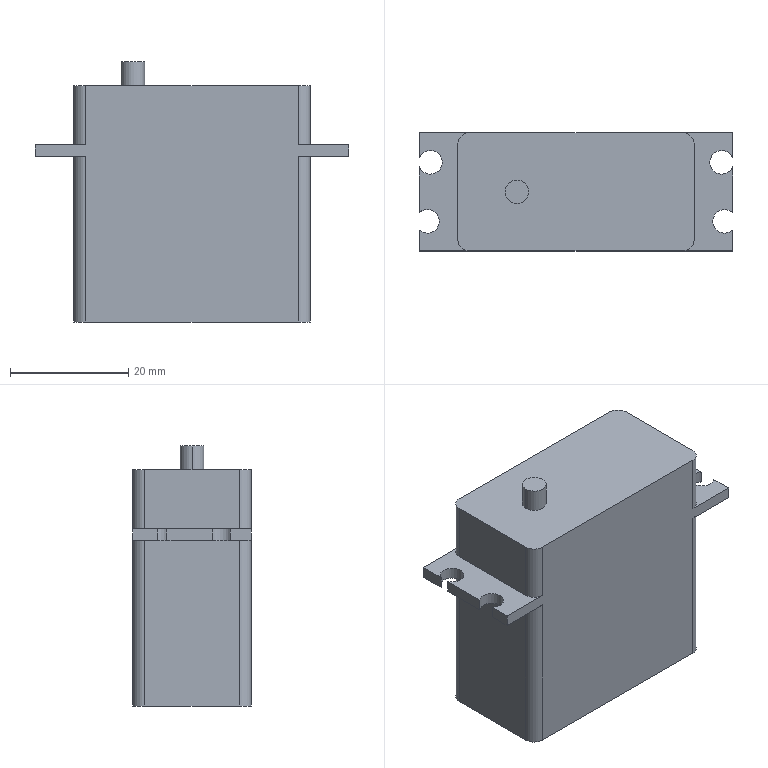Part | SolidWorks | features ICE 3, Extrusion 1, Fillet 1, MirrorPattern 1 | 1 solid | 35 faces | box 53 x 20 x 44 mm | volume 32345 mm3 | plane 19 | cylinder 16 | commonest cylinder face diameters 4 x16
STEP:
#1=CARTESIAN_POINT('',(-8.,10.,24.));
#2=VERTEX_POINT('',#1);
#3=CARTESIAN_POINT('',(-12.,10.,24.));
#4=VERTEX_POINT('',#3);
#5=CARTESIAN_POINT('',(-10.,10.,24.));
#6=DIRECTION('',(0.,0.,1.));
#7=DIRECTION('',(1.,0.,0.));
#8=AXIS2_PLACEMENT_3D('',#5,#6,#7);
#9=CIRCLE('',#8,2.);
#10=EDGE_CURVE('',#2,#4,#9,.T.);
#11=ORIENTED_EDGE('',*,*,#10,.F.);
#12=CARTESIAN_POINT('',(-8.,10.,20.));
#13=VERTEX_POINT('',#12);
#14=CARTESIAN_POINT('',(-8.,10.,24.));
#15=DIRECTION('',(0.,0.,-1.));
#16=VECTOR('',#15,1000.);
#17=LINE('',#14,#16);
#18=EDGE_CURVE('',#2,#13,#17,.T.);
#19=ORIENTED_EDGE('',*,*,#18,.T.);
#20=CARTESIAN_POINT('',(-12.,10.,20.));
#21=VERTEX_POINT('',#20);
#22=CARTESIAN_POINT('',(-10.,10.,20.));
#23=DIRECTION('',(0.,0.,1.));
#24=DIRECTION('',(-1.,0.,0.));
#25=AXIS2_PLACEMENT_3D('',#22,#23,#24);
#26=CIRCLE('',#25,2.);
#27=EDGE_CURVE('',#13,#21,#26,.T.);
#28=ORIENTED_EDGE('',*,*,#27,.T.);
#29=CARTESIAN_POINT('',(-12.,10.,24.));
#30=DIRECTION('',(0.,0.,-1.));
#31=VECTOR('',#30,1000.);
#32=LINE('',#29,#31);
#33=EDGE_CURVE('',#4,#21,#32,.T.);
#34=ORIENTED_EDGE('',*,*,#33,.F.);
#35=EDGE_LOOP('',(#11,#19,#28,#34));
#36=FACE_OUTER_BOUND('',#35,.T.);
#37=CARTESIAN_POINT('',(-10.,10.,24.));
#38=DIRECTION('',(0.,0.,-1.));
#39=DIRECTION('',(-1.,0.,0.));
#40=AXIS2_PLACEMENT_3D('',#37,#38,#39);
#41=CYLINDRICAL_SURFACE('',#40,2.);
#42=ADVANCED_FACE('',(#36),#41,.T.);
#43=CARTESIAN_POINT('',(26.5,15.76,10.));
#44=VERTEX_POINT('',#43);
#45=CARTESIAN_POINT('',(22.65,15.,10.));
#46=VERTEX_POINT('',#45);
#47=CARTESIAN_POINT('',(24.65,15.,10.));
#48=DIRECTION('',(0.,0.,1.));
#49=DIRECTION('',(1.,0.,0.));
#50=AXIS2_PLACEMENT_3D('',#47,#48,#49);
#51=CIRCLE('',#50,2.);
#52=EDGE_CURVE('',#44,#46,#51,.T.);
#53=ORIENTED_EDGE('',*,*,#52,.T.);
#54=CARTESIAN_POINT('',(22.65,15.,8.));
#55=VERTEX_POINT('',#54);
#56=CARTESIAN_POINT('',(22.65,15.,10.));
#57=DIRECTION('',(0.,0.,-1.));
#58=VECTOR('',#57,1000.);
#59=LINE('',#56,#58);
#60=EDGE_CURVE('',#46,#55,#59,.T.);
#61=ORIENTED_EDGE('',*,*,#60,.T.);
#62=CARTESIAN_POINT('',(26.5,15.76,8.));
#63=VERTEX_POINT('',#62);
#64=CARTESIAN_POINT('',(24.65,15.,8.));
#65=DIRECTION('',(0.,0.,1.));
#66=DIRECTION('',(1.,0.,0.));
#67=AXIS2_PLACEMENT_3D('',#64,#65,#66);
#68=CIRCLE('',#67,2.);
#69=EDGE_CURVE('',#63,#55,#68,.T.);
#70=ORIENTED_EDGE('',*,*,#69,.F.);
#71=CARTESIAN_POINT('',(26.5,15.76,10.));
#72=DIRECTION('',(0.,0.,-1.));
#73=VECTOR('',#72,1000.);
#74=LINE('',#71,#73);
#75=EDGE_CURVE('',#44,#63,#74,.T.);
#76=ORIENTED_EDGE('',*,*,#75,.F.);
#77=EDGE_LOOP('',(#53,#61,#70,#76));
#78=FACE_OUTER_BOUND('',#77,.T.);
#79=CARTESIAN_POINT('',(24.65,15.,10.));
#80=DIRECTION('',(0.,0.,-1.));
#81=DIRECTION('',(-1.,0.,0.));
#82=AXIS2_PLACEMENT_3D('',#79,#80,#81);
#83=CYLINDRICAL_SURFACE('',#82,2.);
#84=ADVANCED_FACE('',(#78),#83,.F.);
#85=CARTESIAN_POINT('',(26.5,6.488,10.));
#86=VERTEX_POINT('',#85);
#87=CARTESIAN_POINT('',(23.149,5.012,10.));
#88=VERTEX_POINT('',#87);
#89=CARTESIAN_POINT('',(25.149,5.012,10.));
#90=DIRECTION('',(0.,0.,1.));
#91=DIRECTION('',(1.,0.,0.));
#92=AXIS2_PLACEMENT_3D('',#89,#90,#91);
#93=CIRCLE('',#92,2.);
#94=EDGE_CURVE('',#86,#88,#93,.T.);
#95=ORIENTED_EDGE('',*,*,#94,.T.);
#96=CARTESIAN_POINT('',(23.149,5.012,8.));
#97=VERTEX_POINT('',#96);
#98=CARTESIAN_POINT('',(23.149,5.012,10.));
#99=DIRECTION('',(0.,0.,-1.));
#100=VECTOR('',#99,1000.);
#101=LINE('',#98,#100);
#102=EDGE_CURVE('',#88,#97,#101,.T.);
#103=ORIENTED_EDGE('',*,*,#102,.T.);
#104=CARTESIAN_POINT('',(26.5,6.488,8.));
#105=VERTEX_POINT('',#104);
#106=CARTESIAN_POINT('',(25.149,5.012,8.));
#107=DIRECTION('',(0.,0.,1.));
#108=DIRECTION('',(1.,0.,0.));
#109=AXIS2_PLACEMENT_3D('',#106,#107,#108);
#110=CIRCLE('',#109,2.);
#111=EDGE_CURVE('',#105,#97,#110,.T.);
#112=ORIENTED_EDGE('',*,*,#111,.F.);
#113=CARTESIAN_POINT('',(26.5,6.488,10.));
#114=DIRECTION('',(0.,0.,-1.));
#115=VECTOR('',#114,1000.);
#116=LINE('',#113,#115);
#117=EDGE_CURVE('',#86,#105,#116,.T.);
#118=ORIENTED_EDGE('',*,*,#117,.F.);
#119=EDGE_LOOP('',(#95,#103,#112,#118));
#120=FACE_OUTER_BOUND('',#119,.T.);
#121=CARTESIAN_POINT('',(25.149,5.012,10.));
#122=DIRECTION('',(0.,0.,-1.));
#123=DIRECTION('',(-1.,0.,0.));
#124=AXIS2_PLACEMENT_3D('',#121,#122,#123);
#125=CYLINDRICAL_SURFACE('',#124,2.);
#126=ADVANCED_FACE('',(#120),#125,.F.);
#127=CARTESIAN_POINT('',(26.5,14.24,8.));
#128=VERTEX_POINT('',#127);
#129=CARTESIAN_POINT('',(26.5,0.,8.));
#130=DIRECTION('',(0.,-1.,0.));
#131=VECTOR('',#130,1000.);
#132=LINE('',#129,#131);
#133=EDGE_CURVE('',#128,#105,#132,.T.);
#134=ORIENTED_EDGE('',*,*,#133,.F.);
#135=CARTESIAN_POINT('',(26.5,14.24,10.));
#136=VERTEX_POINT('',#135);
#137=CARTESIAN_POINT('',(26.5,14.24,10.));
#138=DIRECTION('',(0.,0.,1.));
#139=VECTOR('',#138,1000.);
#140=LINE('',#137,#139);
#141=EDGE_CURVE('',#128,#136,#140,.T.);
#142=ORIENTED_EDGE('',*,*,#141,.T.);
#143=CARTESIAN_POINT('',(26.5,0.,10.));
#144=DIRECTION('',(0.,-1.,0.));
#145=VECTOR('',#144,1000.);
#146=LINE('',#143,#145);
#147=EDGE_CURVE('',#136,#86,#146,.T.);
#148=ORIENTED_EDGE('',*,*,#147,.T.);
#149=ORIENTED_EDGE('',*,*,#117,.T.);
#150=EDGE_LOOP('',(#134,#142,#148,#149));
#151=FACE_OUTER_BOUND('',#150,.T.);
#152=CARTESIAN_POINT('',(26.5,0.,10.));
#153=DIRECTION('',(1.,0.,0.));
#154=DIRECTION('',(0.,1.,0.));
#155=AXIS2_PLACEMENT_3D('',#152,#153,#154);
#156=PLANE('',#155);
#157=ADVANCED_FACE('',(#151),#156,.T.);
#158=CARTESIAN_POINT('',(26.5,20.,10.));
#159=VERTEX_POINT('',#158);
#160=CARTESIAN_POINT('',(26.5,0.,10.));
#161=DIRECTION('',(0.,-1.,0.));
#162=VECTOR('',#161,1000.);
#163=LINE('',#160,#162);
#164=EDGE_CURVE('',#159,#44,#163,.T.);
#165=ORIENTED_EDGE('',*,*,#164,.T.);
#166=ORIENTED_EDGE('',*,*,#75,.T.);
#167=CARTESIAN_POINT('',(26.5,20.,8.));
#168=VERTEX_POINT('',#167);
#169=CARTESIAN_POINT('',(26.5,0.,8.));
#170=DIRECTION('',(0.,-1.,0.));
#171=VECTOR('',#170,1000.);
#172=LINE('',#169,#171);
#173=EDGE_CURVE('',#168,#63,#172,.T.);
#174=ORIENTED_EDGE('',*,*,#173,.F.);
#175=CARTESIAN_POINT('',(26.5,20.,10.));
#176=DIRECTION('',(0.,0.,-1.));
#177=VECTOR('',#176,1000.);
#178=LINE('',#175,#177);
#179=EDGE_CURVE('',#159,#168,#178,.T.);
#180=ORIENTED_EDGE('',*,*,#179,.F.);
#181=EDGE_LOOP('',(#165,#166,#174,#180));
#182=FACE_OUTER_BOUND('',#181,.T.);
#183=CARTESIAN_POINT('',(26.5,0.,10.));
#184=DIRECTION('',(1.,0.,0.));
#185=DIRECTION('',(0.,1.,0.));
#186=AXIS2_PLACEMENT_3D('',#183,#184,#185);
#187=PLANE('',#186);
#188=ADVANCED_FACE('',(#182),#187,.T.);
#189=CARTESIAN_POINT('',(26.5,3.537,8.));
#190=VERTEX_POINT('',#189);
#191=CARTESIAN_POINT('',(26.5,0.,8.));
#192=VERTEX_POINT('',#191);
#193=CARTESIAN_POINT('',(26.5,0.,8.));
#194=DIRECTION('',(0.,-1.,0.));
#195=VECTOR('',#194,1000.);
#196=LINE('',#193,#195);
#197=EDGE_CURVE('',#190,#192,#196,.T.);
#198=ORIENTED_EDGE('',*,*,#197,.F.);
#199=CARTESIAN_POINT('',(26.5,3.537,10.));
#200=VERTEX_POINT('',#199);
#201=CARTESIAN_POINT('',(26.5,3.537,10.));
#202=DIRECTION('',(0.,0.,1.));
#203=VECTOR('',#202,1000.);
#204=LINE('',#201,#203);
#205=EDGE_CURVE('',#190,#200,#204,.T.);
#206=ORIENTED_EDGE('',*,*,#205,.T.);
#207=CARTESIAN_POINT('',(26.5,0.,10.));
#208=VERTEX_POINT('',#207);
#209=CARTESIAN_POINT('',(26.5,0.,10.));
#210=DIRECTION('',(0.,-1.,0.));
#211=VECTOR('',#210,1000.);
#212=LINE('',#209,#211);
#213=EDGE_CURVE('',#200,#208,#212,.T.);
#214=ORIENTED_EDGE('',*,*,#213,.T.);
#215=CARTESIAN_POINT('',(26.5,0.,10.));
#216=DIRECTION('',(0.,0.,-1.));
#217=VECTOR('',#216,1000.);
#218=LINE('',#215,#217);
#219=EDGE_CURVE('',#208,#192,#218,.T.);
#220=ORIENTED_EDGE('',*,*,#219,.T.);
#221=EDGE_LOOP('',(#198,#206,#214,#220));
#222=FACE_OUTER_BOUND('',#221,.T.);
#223=CARTESIAN_POINT('',(26.5,0.,10.));
#224=DIRECTION('',(1.,0.,0.));
#225=DIRECTION('',(0.,1.,0.));
#226=AXIS2_PLACEMENT_3D('',#223,#224,#225);
#227=PLANE('',#226);
#228=ADVANCED_FACE('',(#222),#227,.T.);
#229=CARTESIAN_POINT('',(-26.5,15.76,10.));
#230=VERTEX_POINT('',#229);
#231=CARTESIAN_POINT('',(-26.5,15.76,8.));
#232=VERTEX_POINT('',#231);
#233=CARTESIAN_POINT('',(-26.5,15.76,10.));
#234=DIRECTION('',(0.,0.,-1.));
#235=VECTOR('',#234,1000.);
#236=LINE('',#233,#235);
#237=EDGE_CURVE('',#230,#232,#236,.T.);
#238=ORIENTED_EDGE('',*,*,#237,.F.);
#239=CARTESIAN_POINT('',(-26.5,20.,10.));
#240=VERTEX_POINT('',#239);
#241=CARTESIAN_POINT('',(-26.5,0.,10.));
#242=DIRECTION('',(0.,1.,0.));
#243=VECTOR('',#242,1000.);
#244=LINE('',#241,#243);
#245=EDGE_CURVE('',#230,#240,#244,.T.);
#246=ORIENTED_EDGE('',*,*,#245,.T.);
#247=CARTESIAN_POINT('',(-26.5,20.,8.));
#248=VERTEX_POINT('',#247);
#249=CARTESIAN_POINT('',(-26.5,20.,10.));
#250=DIRECTION('',(0.,0.,-1.));
#251=VECTOR('',#250,1000.);
#252=LINE('',#249,#251);
#253=EDGE_CURVE('',#240,#248,#252,.T.);
#254=ORIENTED_EDGE('',*,*,#253,.T.);
#255=CARTESIAN_POINT('',(-26.5,0.,8.));
#256=DIRECTION('',(0.,1.,0.));
#257=VECTOR('',#256,1000.);
#258=LINE('',#255,#257);
#259=EDGE_CURVE('',#232,#248,#258,.T.);
#260=ORIENTED_EDGE('',*,*,#259,.F.);
#261=EDGE_LOOP('',(#238,#246,#254,#260));
#262=FACE_OUTER_BOUND('',#261,.T.);
#263=CARTESIAN_POINT('',(-26.5,0.,10.));
#264=DIRECTION('',(-1.,0.,0.));
#265=DIRECTION('',(0.,0.,1.));
#266=AXIS2_PLACEMENT_3D('',#263,#264,#265);
#267=PLANE('',#266);
#268=ADVANCED_FACE('',(#262),#267,.T.);
#269=CARTESIAN_POINT('',(-26.5,14.24,8.));
#270=VERTEX_POINT('',#269);
#271=CARTESIAN_POINT('',(-26.5,14.24,10.));
#272=VERTEX_POINT('',#271);
#273=CARTESIAN_POINT('',(-26.5,14.24,10.));
#274=DIRECTION('',(0.,0.,1.));
#275=VECTOR('',#274,1000.);
#276=LINE('',#273,#275);
#277=EDGE_CURVE('',#270,#272,#276,.T.);
#278=ORIENTED_EDGE('',*,*,#277,.F.);
#279=CARTESIAN_POINT('',(-26.5,6.488,8.));
#280=VERTEX_POINT('',#279);
#281=CARTESIAN_POINT('',(-26.5,0.,8.));
#282=DIRECTION('',(0.,1.,0.));
#283=VECTOR('',#282,1000.);
#284=LINE('',#281,#283);
#285=EDGE_CURVE('',#280,#270,#284,.T.);
#286=ORIENTED_EDGE('',*,*,#285,.F.);
#287=CARTESIAN_POINT('',(-26.5,6.488,10.));
#288=VERTEX_POINT('',#287);
#289=CARTESIAN_POINT('',(-26.5,6.488,10.));
#290=DIRECTION('',(0.,0.,-1.));
#291=VECTOR('',#290,1000.);
#292=LINE('',#289,#291);
#293=EDGE_CURVE('',#288,#280,#292,.T.);
#294=ORIENTED_EDGE('',*,*,#293,.F.);
#295=CARTESIAN_POINT('',(-26.5,0.,10.));
#296=DIRECTION('',(0.,1.,0.));
#297=VECTOR('',#296,1000.);
#298=LINE('',#295,#297);
#299=EDGE_CURVE('',#288,#272,#298,.T.);
#300=ORIENTED_EDGE('',*,*,#299,.T.);
#301=EDGE_LOOP('',(#278,#286,#294,#300));
#302=FACE_OUTER_BOUND('',#301,.T.);
#303=CARTESIAN_POINT('',(-26.5,0.,10.));
#304=DIRECTION('',(-1.,0.,0.));
#305=DIRECTION('',(0.,0.,1.));
#306=AXIS2_PLACEMENT_3D('',#303,#304,#305);
#307=PLANE('',#306);
#308=ADVANCED_FACE('',(#302),#307,.T.);
#309=CARTESIAN_POINT('',(20.,18.,10.));
#310=VERTEX_POINT('',#309);
#311=CARTESIAN_POINT('',(20.,2.,10.));
#312=VERTEX_POINT('',#311);
#313=CARTESIAN_POINT('',(20.,0.,10.));
#314=DIRECTION('',(0.,-1.,0.));
#315=VECTOR('',#314,1000.);
#316=LINE('',#313,#315);
#317=EDGE_CURVE('',#310,#312,#316,.T.);
#318=ORIENTED_EDGE('',*,*,#317,.F.);
#319=CARTESIAN_POINT('',(20.,18.,20.));
#320=VERTEX_POINT('',#319);
#321=CARTESIAN_POINT('',(20.,18.,20.));
#322=DIRECTION('',(0.,0.,1.));
#323=VECTOR('',#322,1000.);
#324=LINE('',#321,#323);
#325=EDGE_CURVE('',#310,#320,#324,.T.);
#326=ORIENTED_EDGE('',*,*,#325,.T.);
#327=CARTESIAN_POINT('',(20.,2.,20.));
#328=VERTEX_POINT('',#327);
#329=CARTESIAN_POINT('',(20.,20.,20.));
#330=DIRECTION('',(0.,-1.,0.));
#331=VECTOR('',#330,1000.);
#332=LINE('',#329,#331);
#333=EDGE_CURVE('',#320,#328,#332,.T.);
#334=ORIENTED_EDGE('',*,*,#333,.T.);
#335=CARTESIAN_POINT('',(20.,2.,10.));
#336=DIRECTION('',(0.,0.,-1.));
#337=VECTOR('',#336,1000.);
#338=LINE('',#335,#337);
#339=EDGE_CURVE('',#328,#312,#338,.T.);
#340=ORIENTED_EDGE('',*,*,#339,.T.);
#341=EDGE_LOOP('',(#318,#326,#334,#340));
#342=FACE_OUTER_BOUND('',#341,.T.);
#343=CARTESIAN_POINT('',(20.,20.,20.));
#344=DIRECTION('',(-1.,0.,0.));
#345=DIRECTION('',(0.,0.,1.));
#346=AXIS2_PLACEMENT_3D('',#343,#344,#345);
#347=PLANE('',#346);
#348=ADVANCED_FACE('',(#342),#347,.F.);
#349=CARTESIAN_POINT('',(-20.,2.,10.));
#350=VERTEX_POINT('',#349);
#351=CARTESIAN_POINT('',(-20.,18.,10.));
#352=VERTEX_POINT('',#351);
#353=CARTESIAN_POINT('',(-20.,0.,10.));
#354=DIRECTION('',(0.,1.,0.));
#355=VECTOR('',#354,1000.);
#356=LINE('',#353,#355);
#357=EDGE_CURVE('',#350,#352,#356,.T.);
#358=ORIENTED_EDGE('',*,*,#357,.F.);
#359=CARTESIAN_POINT('',(-20.,2.,20.));
#360=VERTEX_POINT('',#359);
#361=CARTESIAN_POINT('',(-20.,2.,20.));
#362=DIRECTION('',(0.,0.,1.));
#363=VECTOR('',#362,1000.);
#364=LINE('',#361,#363);
#365=EDGE_CURVE('',#350,#360,#364,.T.);
#366=ORIENTED_EDGE('',*,*,#365,.T.);
#367=CARTESIAN_POINT('',(-20.,18.,20.));
#368=VERTEX_POINT('',#367);
#369=CARTESIAN_POINT('',(-20.,20.,20.));
#370=DIRECTION('',(0.,-1.,0.));
#371=VECTOR('',#370,1000.);
#372=LINE('',#369,#371);
#373=EDGE_CURVE('',#368,#360,#372,.T.);
#374=ORIENTED_EDGE('',*,*,#373,.F.);
#375=CARTESIAN_POINT('',(-20.,18.,20.));
#376=DIRECTION('',(0.,0.,-1.));
#377=VECTOR('',#376,1000.);
#378=LINE('',#375,#377);
#379=EDGE_CURVE('',#368,#352,#378,.T.);
#380=ORIENTED_EDGE('',*,*,#379,.T.);
#381=EDGE_LOOP('',(#358,#366,#374,#380));
#382=FACE_OUTER_BOUND('',#381,.T.);
#383=CARTESIAN_POINT('',(-20.,20.,20.));
#384=DIRECTION('',(1.,0.,0.));
#385=DIRECTION('',(0.,0.,-1.));
#386=AXIS2_PLACEMENT_3D('',#383,#384,#385);
#387=PLANE('',#386);
#388=ADVANCED_FACE('',(#382),#387,.F.);
#389=CARTESIAN_POINT('',(20.,18.,-20.));
#390=VERTEX_POINT('',#389);
#391=CARTESIAN_POINT('',(20.,2.,-20.));
#392=VERTEX_POINT('',#391);
#393=CARTESIAN_POINT('',(20.,20.,-20.));
#394=DIRECTION('',(0.,-1.,0.));
#395=VECTOR('',#394,1000.);
#396=LINE('',#393,#395);
#397=EDGE_CURVE('',#390,#392,#396,.T.);
#398=ORIENTED_EDGE('',*,*,#397,.F.);
#399=CARTESIAN_POINT('',(20.,18.,8.));
#400=VERTEX_POINT('',#399);
#401=CARTESIAN_POINT('',(20.,18.,20.));
#402=DIRECTION('',(0.,0.,1.));
#403=VECTOR('',#402,1000.);
#404=LINE('',#401,#403);
#405=EDGE_CURVE('',#390,#400,#404,.T.);
#406=ORIENTED_EDGE('',*,*,#405,.T.);
#407=CARTESIAN_POINT('',(20.,2.,8.));
#408=VERTEX_POINT('',#407);
#409=CARTESIAN_POINT('',(20.,0.,8.));
#410=DIRECTION('',(0.,-1.,0.));
#411=VECTOR('',#410,1000.);
#412=LINE('',#409,#411);
#413=EDGE_CURVE('',#400,#408,#412,.T.);
#414=ORIENTED_EDGE('',*,*,#413,.T.);
#415=CARTESIAN_POINT('',(20.,2.,-20.));
#416=DIRECTION('',(0.,0.,-1.));
#417=VECTOR('',#416,1000.);
#418=LINE('',#415,#417);
#419=EDGE_CURVE('',#408,#392,#418,.T.);
#420=ORIENTED_EDGE('',*,*,#419,.T.);
#421=EDGE_LOOP('',(#398,#406,#414,#420));
#422=FACE_OUTER_BOUND('',#421,.T.);
#423=CARTESIAN_POINT('',(20.,20.,20.));
#424=DIRECTION('',(-1.,0.,0.));
#425=DIRECTION('',(0.,0.,1.));
#426=AXIS2_PLACEMENT_3D('',#423,#424,#425);
#427=PLANE('',#426);
#428=ADVANCED_FACE('',(#422),#427,.F.);
#429=CARTESIAN_POINT('',(18.,20.,-20.));
#430=VERTEX_POINT('',#429);
#431=CARTESIAN_POINT('',(-18.,20.,-20.));
#432=VERTEX_POINT('',#431);
#433=CARTESIAN_POINT('',(-20.,20.,-20.));
#434=DIRECTION('',(-1.,0.,0.));
#435=VECTOR('',#434,1000.);
#436=LINE('',#433,#435);
#437=EDGE_CURVE('',#430,#432,#436,.T.);
#438=ORIENTED_EDGE('',*,*,#437,.F.);
#439=CARTESIAN_POINT('',(18.,18.,-20.));
#440=DIRECTION('',(0.,0.,-1.));
#441=DIRECTION('',(1.,0.,0.));
#442=AXIS2_PLACEMENT_3D('',#439,#440,#441);
#443=CIRCLE('',#442,2.);
#444=EDGE_CURVE('',#430,#390,#443,.T.);
#445=ORIENTED_EDGE('',*,*,#444,.T.);
#446=ORIENTED_EDGE('',*,*,#397,.T.);
#447=CARTESIAN_POINT('',(18.,0.,-20.));
#448=VERTEX_POINT('',#447);
#449=CARTESIAN_POINT('',(18.,2.,-20.));
#450=DIRECTION('',(0.,0.,-1.));
#451=DIRECTION('',(1.,0.,0.));
#452=AXIS2_PLACEMENT_3D('',#449,#450,#451);
#453=CIRCLE('',#452,2.);
#454=EDGE_CURVE('',#392,#448,#453,.T.);
#455=ORIENTED_EDGE('',*,*,#454,.T.);
#456=CARTESIAN_POINT('',(-18.,0.,-20.));
#457=VERTEX_POINT('',#456);
#458=CARTESIAN_POINT('',(-20.,0.,-20.));
#459=DIRECTION('',(-1.,0.,0.));
#460=VECTOR('',#459,1000.);
#461=LINE('',#458,#460);
#462=EDGE_CURVE('',#448,#457,#461,.T.);
#463=ORIENTED_EDGE('',*,*,#462,.T.);
#464=CARTESIAN_POINT('',(-20.,2.,-20.));
#465=VERTEX_POINT('',#464);
#466=CARTESIAN_POINT('',(-18.,2.,-20.));
#467=DIRECTION('',(0.,0.,-1.));
#468=DIRECTION('',(1.,0.,0.));
#469=AXIS2_PLACEMENT_3D('',#466,#467,#468);
#470=CIRCLE('',#469,2.);
#471=EDGE_CURVE('',#457,#465,#470,.T.);
#472=ORIENTED_EDGE('',*,*,#471,.T.);
#473=CARTESIAN_POINT('',(-20.,18.,-20.));
#474=VERTEX_POINT('',#473);
#475=CARTESIAN_POINT('',(-20.,20.,-20.));
#476=DIRECTION('',(0.,-1.,0.));
#477=VECTOR('',#476,1000.);
#478=LINE('',#475,#477);
#479=EDGE_CURVE('',#474,#465,#478,.T.);
#480=ORIENTED_EDGE('',*,*,#479,.F.);
#481=CARTESIAN_POINT('',(-18.,18.,-20.));
#482=DIRECTION('',(0.,0.,-1.));
#483=DIRECTION('',(1.,0.,0.));
#484=AXIS2_PLACEMENT_3D('',#481,#482,#483);
#485=CIRCLE('',#484,2.);
#486=EDGE_CURVE('',#474,#432,#485,.T.);
#487=ORIENTED_EDGE('',*,*,#486,.T.);
#488=EDGE_LOOP('',(#438,#445,#446,#455,#463,#472,#480,#487));
#489=FACE_OUTER_BOUND('',#488,.T.);
#490=CARTESIAN_POINT('',(-20.,20.,-20.));
#491=DIRECTION('',(0.,0.,1.));
#492=DIRECTION('',(1.,0.,0.));
#493=AXIS2_PLACEMENT_3D('',#490,#491,#492);
#494=PLANE('',#493);
#495=ADVANCED_FACE('',(#489),#494,.F.);
#496=ORIENTED_EDGE('',*,*,#479,.T.);
#497=CARTESIAN_POINT('',(-20.,2.,8.));
#498=VERTEX_POINT('',#497);
#499=CARTESIAN_POINT('',(-20.,2.,8.));
#500=DIRECTION('',(0.,0.,1.));
#501=VECTOR('',#500,1000.);
#502=LINE('',#499,#501);
#503=EDGE_CURVE('',#465,#498,#502,.T.);
#504=ORIENTED_EDGE('',*,*,#503,.T.);
#505=CARTESIAN_POINT('',(-20.,18.,8.));
#506=VERTEX_POINT('',#505);
#507=CARTESIAN_POINT('',(-20.,0.,8.));
#508=DIRECTION('',(0.,1.,0.));
#509=VECTOR('',#508,1000.);
#510=LINE('',#507,#509);
#511=EDGE_CURVE('',#498,#506,#510,.T.);
#512=ORIENTED_EDGE('',*,*,#511,.T.);
#513=CARTESIAN_POINT('',(-20.,18.,20.));
#514=DIRECTION('',(0.,0.,-1.));
#515=VECTOR('',#514,1000.);
#516=LINE('',#513,#515);
#517=EDGE_CURVE('',#506,#474,#516,.T.);
#518=ORIENTED_EDGE('',*,*,#517,.T.);
#519=EDGE_LOOP('',(#496,#504,#512,#518));
#520=FACE_OUTER_BOUND('',#519,.T.);
#521=CARTESIAN_POINT('',(-20.,20.,20.));
#522=DIRECTION('',(1.,0.,0.));
#523=DIRECTION('',(0.,0.,-1.));
#524=AXIS2_PLACEMENT_3D('',#521,#522,#523);
#525=PLANE('',#524);
#526=ADVANCED_FACE('',(#520),#525,.F.);
#527=CARTESIAN_POINT('',(-10.,10.,20.));
#528=DIRECTION('',(0.,0.,1.));
#529=DIRECTION('',(-1.,0.,0.));
#530=AXIS2_PLACEMENT_3D('',#527,#528,#529);
#531=CIRCLE('',#530,2.);
#532=EDGE_CURVE('',#21,#13,#531,.T.);
#533=ORIENTED_EDGE('',*,*,#532,.F.);
#534=ORIENTED_EDGE('',*,*,#27,.F.);
#535=EDGE_LOOP('',(#533,#534));
#536=FACE_BOUND('',#535,.T.);
#537=ORIENTED_EDGE('',*,*,#333,.F.);
#538=CARTESIAN_POINT('',(18.,20.,20.));
#539=VERTEX_POINT('',#538);
#540=CARTESIAN_POINT('',(18.,18.,20.));
#541=DIRECTION('',(0.,0.,1.));
#542=DIRECTION('',(-1.,0.,0.));
#543=AXIS2_PLACEMENT_3D('',#540,#541,#542);
#544=CIRCLE('',#543,2.);
#545=EDGE_CURVE('',#320,#539,#544,.T.);
#546=ORIENTED_EDGE('',*,*,#545,.T.);
#547=CARTESIAN_POINT('',(-18.,20.,20.));
#548=VERTEX_POINT('',#547);
#549=CARTESIAN_POINT('',(-20.,20.,20.));
#550=DIRECTION('',(1.,0.,0.));
#551=VECTOR('',#550,1000.);
#552=LINE('',#549,#551);
#553=EDGE_CURVE('',#548,#539,#552,.T.);
#554=ORIENTED_EDGE('',*,*,#553,.F.);
#555=CARTESIAN_POINT('',(-18.,18.,20.));
#556=DIRECTION('',(0.,0.,1.));
#557=DIRECTION('',(-1.,0.,0.));
#558=AXIS2_PLACEMENT_3D('',#555,#556,#557);
#559=CIRCLE('',#558,2.);
#560=EDGE_CURVE('',#548,#368,#559,.T.);
#561=ORIENTED_EDGE('',*,*,#560,.T.);
#562=ORIENTED_EDGE('',*,*,#373,.T.);
#563=CARTESIAN_POINT('',(-18.,0.,20.));
#564=VERTEX_POINT('',#563);
#565=CARTESIAN_POINT('',(-18.,2.,20.));
#566=DIRECTION('',(0.,0.,1.));
#567=DIRECTION('',(-1.,0.,0.));
#568=AXIS2_PLACEMENT_3D('',#565,#566,#567);
#569=CIRCLE('',#568,2.);
#570=EDGE_CURVE('',#360,#564,#569,.T.);
#571=ORIENTED_EDGE('',*,*,#570,.T.);
#572=CARTESIAN_POINT('',(18.,0.,20.));
#573=VERTEX_POINT('',#572);
#574=CARTESIAN_POINT('',(-20.,0.,20.));
#575=DIRECTION('',(1.,0.,0.));
#576=VECTOR('',#575,1000.);
#577=LINE('',#574,#576);
#578=EDGE_CURVE('',#564,#573,#577,.T.);
#579=ORIENTED_EDGE('',*,*,#578,.T.);
#580=CARTESIAN_POINT('',(18.,2.,20.));
#581=DIRECTION('',(0.,0.,1.));
#582=DIRECTION('',(-1.,0.,0.));
#583=AXIS2_PLACEMENT_3D('',#580,#581,#582);
#584=CIRCLE('',#583,2.);
#585=EDGE_CURVE('',#573,#328,#584,.T.);
#586=ORIENTED_EDGE('',*,*,#585,.T.);
#587=EDGE_LOOP('',(#537,#546,#554,#561,#562,#571,#579,#586));
#588=FACE_OUTER_BOUND('',#587,.T.);
#589=CARTESIAN_POINT('',(-20.,20.,20.));
#590=DIRECTION('',(0.,0.,-1.));
#591=DIRECTION('',(-1.,0.,0.));
#592=AXIS2_PLACEMENT_3D('',#589,#590,#591);
#593=PLANE('',#592);
#594=ADVANCED_FACE('',(#536,#588),#593,.F.);
#595=CARTESIAN_POINT('',(18.,20.,8.));
#596=VERTEX_POINT('',#595);
#597=CARTESIAN_POINT('',(0.,20.,8.));
#598=DIRECTION('',(1.,0.,0.));
#599=VECTOR('',#598,1000.);
#600=LINE('',#597,#599);
#601=EDGE_CURVE('',#596,#168,#600,.T.);
#602=ORIENTED_EDGE('',*,*,#601,.F.);
#603=CARTESIAN_POINT('',(18.,20.,0.));
#604=DIRECTION('',(0.,0.,-1.));
#605=VECTOR('',#604,1000.);
#606=LINE('',#603,#605);
#607=EDGE_CURVE('',#596,#430,#606,.T.);
#608=ORIENTED_EDGE('',*,*,#607,.T.);
#609=ORIENTED_EDGE('',*,*,#437,.T.);
#610=CARTESIAN_POINT('',(-18.,20.,8.));
#611=VERTEX_POINT('',#610);
#612=CARTESIAN_POINT('',(-18.,20.,0.));
#613=DIRECTION('',(0.,0.,1.));
#614=VECTOR('',#613,1000.);
#615=LINE('',#612,#614);
#616=EDGE_CURVE('',#432,#611,#615,.T.);
#617=ORIENTED_EDGE('',*,*,#616,.T.);
#618=CARTESIAN_POINT('',(0.,20.,8.));
#619=DIRECTION('',(-1.,0.,0.));
#620=VECTOR('',#619,1000.);
#621=LINE('',#618,#620);
#622=EDGE_CURVE('',#611,#248,#621,.T.);
#623=ORIENTED_EDGE('',*,*,#622,.T.);
#624=ORIENTED_EDGE('',*,*,#253,.F.);
#625=CARTESIAN_POINT('',(-18.,20.,10.));
#626=VERTEX_POINT('',#625);
#627=CARTESIAN_POINT('',(0.,20.,10.));
#628=DIRECTION('',(-1.,0.,0.));
#629=VECTOR('',#628,1000.);
#630=LINE('',#627,#629);
#631=EDGE_CURVE('',#626,#240,#630,.T.);
#632=ORIENTED_EDGE('',*,*,#631,.F.);
#633=CARTESIAN_POINT('',(-18.,20.,0.));
#634=DIRECTION('',(0.,0.,1.));
#635=VECTOR('',#634,1000.);
#636=LINE('',#633,#635);
#637=EDGE_CURVE('',#626,#548,#636,.T.);
#638=ORIENTED_EDGE('',*,*,#637,.T.);
#639=ORIENTED_EDGE('',*,*,#553,.T.);
#640=CARTESIAN_POINT('',(18.,20.,10.));
#641=VERTEX_POINT('',#640);
#642=CARTESIAN_POINT('',(18.,20.,0.));
#643=DIRECTION('',(0.,0.,-1.));
#644=VECTOR('',#643,1000.);
#645=LINE('',#642,#644);
#646=EDGE_CURVE('',#539,#641,#645,.T.);
#647=ORIENTED_EDGE('',*,*,#646,.T.);
#648=CARTESIAN_POINT('',(0.,20.,10.));
#649=DIRECTION('',(1.,0.,0.));
#650=VECTOR('',#649,1000.);
#651=LINE('',#648,#650);
#652=EDGE_CURVE('',#641,#159,#651,.T.);
#653=ORIENTED_EDGE('',*,*,#652,.T.);
#654=ORIENTED_EDGE('',*,*,#179,.T.);
#655=EDGE_LOOP('',(#602,#608,#609,#617,#623,#624,#632,#638,#639,#647,#653,#654));
#656=FACE_OUTER_BOUND('',#655,.T.);
#657=CARTESIAN_POINT('',(0.,20.,0.));
#658=DIRECTION('',(0.,-1.,0.));
#659=DIRECTION('',(0.,0.,-1.));
#660=AXIS2_PLACEMENT_3D('',#657,#658,#659);
#661=PLANE('',#660);
#662=ADVANCED_FACE('',(#656),#661,.F.);
#663=ORIENTED_EDGE('',*,*,#462,.F.);
#664=CARTESIAN_POINT('',(18.,0.,8.));
#665=VERTEX_POINT('',#664);
#666=CARTESIAN_POINT('',(18.,0.,8.));
#667=DIRECTION('',(0.,0.,1.));
#668=VECTOR('',#667,1000.);
#669=LINE('',#666,#668);
#670=EDGE_CURVE('',#448,#665,#669,.T.);
#671=ORIENTED_EDGE('',*,*,#670,.T.);
#672=CARTESIAN_POINT('',(0.,0.,8.));
#673=DIRECTION('',(1.,0.,0.));
#674=VECTOR('',#673,1000.);
#675=LINE('',#672,#674);
#676=EDGE_CURVE('',#665,#192,#675,.T.);
#677=ORIENTED_EDGE('',*,*,#676,.T.);
#678=ORIENTED_EDGE('',*,*,#219,.F.);
#679=CARTESIAN_POINT('',(18.,0.,10.));
#680=VERTEX_POINT('',#679);
#681=CARTESIAN_POINT('',(0.,0.,10.));
#682=DIRECTION('',(1.,0.,0.));
#683=VECTOR('',#682,1000.);
#684=LINE('',#681,#683);
#685=EDGE_CURVE('',#680,#208,#684,.T.);
#686=ORIENTED_EDGE('',*,*,#685,.F.);
#687=CARTESIAN_POINT('',(18.,0.,20.));
#688=DIRECTION('',(0.,0.,1.));
#689=VECTOR('',#688,1000.);
#690=LINE('',#687,#689);
#691=EDGE_CURVE('',#680,#573,#690,.T.);
#692=ORIENTED_EDGE('',*,*,#691,.T.);
#693=ORIENTED_EDGE('',*,*,#578,.F.);
#694=CARTESIAN_POINT('',(-18.,0.,10.));
#695=VERTEX_POINT('',#694);
#696=CARTESIAN_POINT('',(-18.,0.,10.));
#697=DIRECTION('',(0.,0.,-1.));
#698=VECTOR('',#697,1000.);
#699=LINE('',#696,#698);
#700=EDGE_CURVE('',#564,#695,#699,.T.);
#701=ORIENTED_EDGE('',*,*,#700,.T.);
#702=CARTESIAN_POINT('',(-26.5,0.,10.));
#703=VERTEX_POINT('',#702);
#704=CARTESIAN_POINT('',(0.,0.,10.));
#705=DIRECTION('',(-1.,0.,0.));
#706=VECTOR('',#705,1000.);
#707=LINE('',#704,#706);
#708=EDGE_CURVE('',#695,#703,#707,.T.);
#709=ORIENTED_EDGE('',*,*,#708,.T.);
#710=CARTESIAN_POINT('',(-26.5,0.,8.));
#711=VERTEX_POINT('',#710);
#712=CARTESIAN_POINT('',(-26.5,0.,10.));
#713=DIRECTION('',(0.,0.,-1.));
#714=VECTOR('',#713,1000.);
#715=LINE('',#712,#714);
#716=EDGE_CURVE('',#703,#711,#715,.T.);
#717=ORIENTED_EDGE('',*,*,#716,.T.);
#718=CARTESIAN_POINT('',(-18.,0.,8.));
#719=VERTEX_POINT('',#718);
#720=CARTESIAN_POINT('',(0.,0.,8.));
#721=DIRECTION('',(-1.,0.,0.));
#722=VECTOR('',#721,1000.);
#723=LINE('',#720,#722);
#724=EDGE_CURVE('',#719,#711,#723,.T.);
#725=ORIENTED_EDGE('',*,*,#724,.F.);
#726=CARTESIAN_POINT('',(-18.,0.,-20.));
#727=DIRECTION('',(0.,0.,-1.));
#728=VECTOR('',#727,1000.);
#729=LINE('',#726,#728);
#730=EDGE_CURVE('',#719,#457,#729,.T.);
#731=ORIENTED_EDGE('',*,*,#730,.T.);
#732=EDGE_LOOP('',(#663,#671,#677,#678,#686,#692,#693,#701,#709,#717,#725,#731));
#733=FACE_OUTER_BOUND('',#732,.T.);
#734=CARTESIAN_POINT('',(0.,0.,0.));
#735=DIRECTION('',(0.,-1.,0.));
#736=DIRECTION('',(0.,0.,-1.));
#737=AXIS2_PLACEMENT_3D('',#734,#735,#736);
#738=PLANE('',#737);
#739=ADVANCED_FACE('',(#733),#738,.T.);
#740=CARTESIAN_POINT('',(-26.5,3.537,8.));
#741=VERTEX_POINT('',#740);
#742=CARTESIAN_POINT('',(-26.5,3.537,10.));
#743=VERTEX_POINT('',#742);
#744=CARTESIAN_POINT('',(-26.5,3.537,10.));
#745=DIRECTION('',(0.,0.,1.));
#746=VECTOR('',#745,1000.);
#747=LINE('',#744,#746);
#748=EDGE_CURVE('',#741,#743,#747,.T.);
#749=ORIENTED_EDGE('',*,*,#748,.F.);
#750=CARTESIAN_POINT('',(-26.5,0.,8.));
#751=DIRECTION('',(0.,1.,0.));
#752=VECTOR('',#751,1000.);
#753=LINE('',#750,#752);
#754=EDGE_CURVE('',#711,#741,#753,.T.);
#755=ORIENTED_EDGE('',*,*,#754,.F.);
#756=ORIENTED_EDGE('',*,*,#716,.F.);
#757=CARTESIAN_POINT('',(-26.5,0.,10.));
#758=DIRECTION('',(0.,1.,0.));
#759=VECTOR('',#758,1000.);
#760=LINE('',#757,#759);
#761=EDGE_CURVE('',#703,#743,#760,.T.);
#762=ORIENTED_EDGE('',*,*,#761,.T.);
#763=EDGE_LOOP('',(#749,#755,#756,#762));
#764=FACE_OUTER_BOUND('',#763,.T.);
#765=CARTESIAN_POINT('',(-26.5,0.,10.));
#766=DIRECTION('',(-1.,0.,0.));
#767=DIRECTION('',(0.,0.,1.));
#768=AXIS2_PLACEMENT_3D('',#765,#766,#767);
#769=PLANE('',#768);
#770=ADVANCED_FACE('',(#764),#769,.T.);
#771=ORIENTED_EDGE('',*,*,#245,.F.);
#772=CARTESIAN_POINT('',(-24.65,15.,10.));
#773=DIRECTION('',(0.,0.,-1.));
#774=DIRECTION('',(-1.,0.,0.));
#775=AXIS2_PLACEMENT_3D('',#772,#773,#774);
#776=CIRCLE('',#775,2.);
#777=EDGE_CURVE('',#230,#272,#776,.T.);
#778=ORIENTED_EDGE('',*,*,#777,.T.);
#779=ORIENTED_EDGE('',*,*,#299,.F.);
#780=CARTESIAN_POINT('',(-25.149,5.012,10.));
#781=DIRECTION('',(0.,0.,-1.));
#782=DIRECTION('',(-1.,0.,0.));
#783=AXIS2_PLACEMENT_3D('',#780,#781,#782);
#784=CIRCLE('',#783,2.);
#785=EDGE_CURVE('',#288,#743,#784,.T.);
#786=ORIENTED_EDGE('',*,*,#785,.T.);
#787=ORIENTED_EDGE('',*,*,#761,.F.);
#788=ORIENTED_EDGE('',*,*,#708,.F.);
#789=CARTESIAN_POINT('',(-18.,2.,10.));
#790=DIRECTION('',(0.,0.,-1.));
#791=DIRECTION('',(-1.,0.,0.));
#792=AXIS2_PLACEMENT_3D('',#789,#790,#791);
#793=CIRCLE('',#792,2.);
#794=EDGE_CURVE('',#695,#350,#793,.T.);
#795=ORIENTED_EDGE('',*,*,#794,.T.);
#796=ORIENTED_EDGE('',*,*,#357,.T.);
#797=CARTESIAN_POINT('',(-18.,18.,10.));
#798=DIRECTION('',(0.,0.,-1.));
#799=DIRECTION('',(-1.,0.,0.));
#800=AXIS2_PLACEMENT_3D('',#797,#798,#799);
#801=CIRCLE('',#800,2.);
#802=EDGE_CURVE('',#352,#626,#801,.T.);
#803=ORIENTED_EDGE('',*,*,#802,.T.);
#804=ORIENTED_EDGE('',*,*,#631,.T.);
#805=EDGE_LOOP('',(#771,#778,#779,#786,#787,#788,#795,#796,#803,#804));
#806=FACE_OUTER_BOUND('',#805,.T.);
#807=CARTESIAN_POINT('',(0.,0.,10.));
#808=DIRECTION('',(0.,0.,-1.));
#809=DIRECTION('',(-1.,0.,0.));
#810=AXIS2_PLACEMENT_3D('',#807,#808,#809);
#811=PLANE('',#810);
#812=ADVANCED_FACE('',(#806),#811,.F.);
#813=CARTESIAN_POINT('',(-24.65,15.,8.));
#814=DIRECTION('',(0.,0.,-1.));
#815=DIRECTION('',(-1.,0.,0.));
#816=AXIS2_PLACEMENT_3D('',#813,#814,#815);
#817=CIRCLE('',#816,2.);
#818=EDGE_CURVE('',#232,#270,#817,.T.);
#819=ORIENTED_EDGE('',*,*,#818,.F.);
#820=ORIENTED_EDGE('',*,*,#259,.T.);
#821=ORIENTED_EDGE('',*,*,#622,.F.);
#822=CARTESIAN_POINT('',(-18.,18.,8.));
#823=DIRECTION('',(0.,0.,1.));
#824=DIRECTION('',(-1.,0.,0.));
#825=AXIS2_PLACEMENT_3D('',#822,#823,#824);
#826=CIRCLE('',#825,2.);
#827=EDGE_CURVE('',#611,#506,#826,.T.);
#828=ORIENTED_EDGE('',*,*,#827,.T.);
#829=ORIENTED_EDGE('',*,*,#511,.F.);
#830=CARTESIAN_POINT('',(-18.,2.,8.));
#831=DIRECTION('',(0.,0.,1.));
#832=DIRECTION('',(-1.,0.,0.));
#833=AXIS2_PLACEMENT_3D('',#830,#831,#832);
#834=CIRCLE('',#833,2.);
#835=EDGE_CURVE('',#498,#719,#834,.T.);
#836=ORIENTED_EDGE('',*,*,#835,.T.);
#837=ORIENTED_EDGE('',*,*,#724,.T.);
#838=ORIENTED_EDGE('',*,*,#754,.T.);
#839=CARTESIAN_POINT('',(-25.149,5.012,8.));
#840=DIRECTION('',(0.,0.,-1.));
#841=DIRECTION('',(-1.,0.,0.));
#842=AXIS2_PLACEMENT_3D('',#839,#840,#841);
#843=CIRCLE('',#842,2.);
#844=EDGE_CURVE('',#280,#741,#843,.T.);
#845=ORIENTED_EDGE('',*,*,#844,.F.);
#846=ORIENTED_EDGE('',*,*,#285,.T.);
#847=EDGE_LOOP('',(#819,#820,#821,#828,#829,#836,#837,#838,#845,#846));
#848=FACE_OUTER_BOUND('',#847,.T.);
#849=CARTESIAN_POINT('',(0.,0.,8.));
#850=DIRECTION('',(0.,0.,-1.));
#851=DIRECTION('',(-1.,0.,0.));
#852=AXIS2_PLACEMENT_3D('',#849,#850,#851);
#853=PLANE('',#852);
#854=ADVANCED_FACE('',(#848),#853,.T.);
#855=ORIENTED_EDGE('',*,*,#52,.F.);
#856=ORIENTED_EDGE('',*,*,#164,.F.);
#857=ORIENTED_EDGE('',*,*,#652,.F.);
#858=CARTESIAN_POINT('',(18.,18.,10.));
#859=DIRECTION('',(0.,0.,-1.));
#860=DIRECTION('',(-1.,0.,0.));
#861=AXIS2_PLACEMENT_3D('',#858,#859,#860);
#862=CIRCLE('',#861,2.);
#863=EDGE_CURVE('',#641,#310,#862,.T.);
#864=ORIENTED_EDGE('',*,*,#863,.T.);
#865=ORIENTED_EDGE('',*,*,#317,.T.);
#866=CARTESIAN_POINT('',(18.,2.,10.));
#867=DIRECTION('',(0.,0.,-1.));
#868=DIRECTION('',(-1.,0.,0.));
#869=AXIS2_PLACEMENT_3D('',#866,#867,#868);
#870=CIRCLE('',#869,2.);
#871=EDGE_CURVE('',#312,#680,#870,.T.);
#872=ORIENTED_EDGE('',*,*,#871,.T.);
#873=ORIENTED_EDGE('',*,*,#685,.T.);
#874=ORIENTED_EDGE('',*,*,#213,.F.);
#875=CARTESIAN_POINT('',(25.149,5.012,10.));
#876=DIRECTION('',(0.,0.,1.));
#877=DIRECTION('',(1.,0.,0.));
#878=AXIS2_PLACEMENT_3D('',#875,#876,#877);
#879=CIRCLE('',#878,2.);
#880=EDGE_CURVE('',#88,#200,#879,.T.);
#881=ORIENTED_EDGE('',*,*,#880,.F.);
#882=ORIENTED_EDGE('',*,*,#94,.F.);
#883=ORIENTED_EDGE('',*,*,#147,.F.);
#884=CARTESIAN_POINT('',(24.65,15.,10.));
#885=DIRECTION('',(0.,0.,1.));
#886=DIRECTION('',(1.,0.,0.));
#887=AXIS2_PLACEMENT_3D('',#884,#885,#886);
#888=CIRCLE('',#887,2.);
#889=EDGE_CURVE('',#46,#136,#888,.T.);
#890=ORIENTED_EDGE('',*,*,#889,.F.);
#891=EDGE_LOOP('',(#855,#856,#857,#864,#865,#872,#873,#874,#881,#882,#883,#890));
#892=FACE_OUTER_BOUND('',#891,.T.);
#893=CARTESIAN_POINT('',(0.,0.,10.));
#894=DIRECTION('',(0.,0.,-1.));
#895=DIRECTION('',(-1.,0.,0.));
#896=AXIS2_PLACEMENT_3D('',#893,#894,#895);
#897=PLANE('',#896);
#898=ADVANCED_FACE('',(#892),#897,.F.);
#899=ORIENTED_EDGE('',*,*,#173,.T.);
#900=ORIENTED_EDGE('',*,*,#69,.T.);
#901=CARTESIAN_POINT('',(24.65,15.,8.));
#902=DIRECTION('',(0.,0.,1.));
#903=DIRECTION('',(1.,0.,0.));
#904=AXIS2_PLACEMENT_3D('',#901,#902,#903);
#905=CIRCLE('',#904,2.);
#906=EDGE_CURVE('',#55,#128,#905,.T.);
#907=ORIENTED_EDGE('',*,*,#906,.T.);
#908=ORIENTED_EDGE('',*,*,#133,.T.);
#909=ORIENTED_EDGE('',*,*,#111,.T.);
#910=CARTESIAN_POINT('',(25.149,5.012,8.));
#911=DIRECTION('',(0.,0.,1.));
#912=DIRECTION('',(1.,0.,0.));
#913=AXIS2_PLACEMENT_3D('',#910,#911,#912);
#914=CIRCLE('',#913,2.);
#915=EDGE_CURVE('',#97,#190,#914,.T.);
#916=ORIENTED_EDGE('',*,*,#915,.T.);
#917=ORIENTED_EDGE('',*,*,#197,.T.);
#918=ORIENTED_EDGE('',*,*,#676,.F.);
#919=CARTESIAN_POINT('',(18.,2.,8.));
#920=DIRECTION('',(0.,0.,1.));
#921=DIRECTION('',(-1.,0.,0.));
#922=AXIS2_PLACEMENT_3D('',#919,#920,#921);
#923=CIRCLE('',#922,2.);
#924=EDGE_CURVE('',#665,#408,#923,.T.);
#925=ORIENTED_EDGE('',*,*,#924,.T.);
#926=ORIENTED_EDGE('',*,*,#413,.F.);
#927=CARTESIAN_POINT('',(18.,18.,8.));
#928=DIRECTION('',(0.,0.,1.));
#929=DIRECTION('',(-1.,0.,0.));
#930=AXIS2_PLACEMENT_3D('',#927,#928,#929);
#931=CIRCLE('',#930,2.);
#932=EDGE_CURVE('',#400,#596,#931,.T.);
#933=ORIENTED_EDGE('',*,*,#932,.T.);
#934=ORIENTED_EDGE('',*,*,#601,.T.);
#935=EDGE_LOOP('',(#899,#900,#907,#908,#909,#916,#917,#918,#925,#926,#933,#934));
#936=FACE_OUTER_BOUND('',#935,.T.);
#937=CARTESIAN_POINT('',(0.,0.,8.));
#938=DIRECTION('',(0.,0.,-1.));
#939=DIRECTION('',(-1.,0.,0.));
#940=AXIS2_PLACEMENT_3D('',#937,#938,#939);
#941=PLANE('',#940);
#942=ADVANCED_FACE('',(#936),#941,.T.);
#943=ORIENTED_EDGE('',*,*,#293,.T.);
#944=ORIENTED_EDGE('',*,*,#844,.T.);
#945=ORIENTED_EDGE('',*,*,#748,.T.);
#946=ORIENTED_EDGE('',*,*,#785,.F.);
#947=EDGE_LOOP('',(#943,#944,#945,#946));
#948=FACE_OUTER_BOUND('',#947,.T.);
#949=CARTESIAN_POINT('',(-25.149,5.012,10.));
#950=DIRECTION('',(0.,0.,-1.));
#951=DIRECTION('',(-1.,0.,0.));
#952=AXIS2_PLACEMENT_3D('',#949,#950,#951);
#953=CYLINDRICAL_SURFACE('',#952,2.);
#954=ADVANCED_FACE('',(#948),#953,.F.);
#955=ORIENTED_EDGE('',*,*,#237,.T.);
#956=ORIENTED_EDGE('',*,*,#818,.T.);
#957=ORIENTED_EDGE('',*,*,#277,.T.);
#958=ORIENTED_EDGE('',*,*,#777,.F.);
#959=EDGE_LOOP('',(#955,#956,#957,#958));
#960=FACE_OUTER_BOUND('',#959,.T.);
#961=CARTESIAN_POINT('',(-24.65,15.,10.));
#962=DIRECTION('',(0.,0.,-1.));
#963=DIRECTION('',(-1.,0.,0.));
#964=AXIS2_PLACEMENT_3D('',#961,#962,#963);
#965=CYLINDRICAL_SURFACE('',#964,2.);
#966=ADVANCED_FACE('',(#960),#965,.F.);
#967=ORIENTED_EDGE('',*,*,#102,.F.);
#968=ORIENTED_EDGE('',*,*,#880,.T.);
#969=ORIENTED_EDGE('',*,*,#205,.F.);
#970=ORIENTED_EDGE('',*,*,#915,.F.);
#971=EDGE_LOOP('',(#967,#968,#969,#970));
#972=FACE_OUTER_BOUND('',#971,.T.);
#973=CARTESIAN_POINT('',(25.149,5.012,10.));
#974=DIRECTION('',(0.,0.,-1.));
#975=DIRECTION('',(-1.,0.,0.));
#976=AXIS2_PLACEMENT_3D('',#973,#974,#975);
#977=CYLINDRICAL_SURFACE('',#976,2.);
#978=ADVANCED_FACE('',(#972),#977,.F.);
#979=ORIENTED_EDGE('',*,*,#60,.F.);
#980=ORIENTED_EDGE('',*,*,#889,.T.);
#981=ORIENTED_EDGE('',*,*,#141,.F.);
#982=ORIENTED_EDGE('',*,*,#906,.F.);
#983=EDGE_LOOP('',(#979,#980,#981,#982));
#984=FACE_OUTER_BOUND('',#983,.T.);
#985=CARTESIAN_POINT('',(24.65,15.,10.));
#986=DIRECTION('',(0.,0.,-1.));
#987=DIRECTION('',(-1.,0.,0.));
#988=AXIS2_PLACEMENT_3D('',#985,#986,#987);
#989=CYLINDRICAL_SURFACE('',#988,2.);
#990=ADVANCED_FACE('',(#984),#989,.F.);
#991=ORIENTED_EDGE('',*,*,#18,.F.);
#992=CARTESIAN_POINT('',(-10.,10.,24.));
#993=DIRECTION('',(0.,0.,1.));
#994=DIRECTION('',(1.,0.,0.));
#995=AXIS2_PLACEMENT_3D('',#992,#993,#994);
#996=CIRCLE('',#995,2.);
#997=EDGE_CURVE('',#4,#2,#996,.T.);
#998=ORIENTED_EDGE('',*,*,#997,.F.);
#999=ORIENTED_EDGE('',*,*,#33,.T.);
#1000=ORIENTED_EDGE('',*,*,#532,.T.);
#1001=EDGE_LOOP('',(#991,#998,#999,#1000));
#1002=FACE_OUTER_BOUND('',#1001,.T.);
#1003=CARTESIAN_POINT('',(-10.,10.,24.));
#1004=DIRECTION('',(0.,0.,-1.));
#1005=DIRECTION('',(-1.,0.,0.));
#1006=AXIS2_PLACEMENT_3D('',#1003,#1004,#1005);
#1007=CYLINDRICAL_SURFACE('',#1006,2.);
#1008=ADVANCED_FACE('',(#1002),#1007,.T.);
#1009=ORIENTED_EDGE('',*,*,#997,.T.);
#1010=ORIENTED_EDGE('',*,*,#10,.T.);
#1011=EDGE_LOOP('',(#1009,#1010));
#1012=FACE_OUTER_BOUND('',#1011,.T.);
#1013=CARTESIAN_POINT('',(-10.,10.,24.));
#1014=DIRECTION('',(0.,0.,1.));
#1015=DIRECTION('',(1.,0.,0.));
#1016=AXIS2_PLACEMENT_3D('',#1013,#1014,#1015);
#1017=PLANE('',#1016);
#1018=ADVANCED_FACE('',(#1012),#1017,.T.);
#1019=ORIENTED_EDGE('',*,*,#932,.F.);
#1020=ORIENTED_EDGE('',*,*,#405,.F.);
#1021=ORIENTED_EDGE('',*,*,#444,.F.);
#1022=ORIENTED_EDGE('',*,*,#607,.F.);
#1023=EDGE_LOOP('',(#1019,#1020,#1021,#1022));
#1024=FACE_OUTER_BOUND('',#1023,.T.);
#1025=CARTESIAN_POINT('',(18.,18.,0.));
#1026=DIRECTION('',(0.,0.,-1.));
#1027=DIRECTION('',(-1.,0.,0.));
#1028=AXIS2_PLACEMENT_3D('',#1025,#1026,#1027);
#1029=CYLINDRICAL_SURFACE('',#1028,2.);
#1030=ADVANCED_FACE('',(#1024),#1029,.T.);
#1031=ORIENTED_EDGE('',*,*,#545,.F.);
#1032=ORIENTED_EDGE('',*,*,#325,.F.);
#1033=ORIENTED_EDGE('',*,*,#863,.F.);
#1034=ORIENTED_EDGE('',*,*,#646,.F.);
#1035=EDGE_LOOP('',(#1031,#1032,#1033,#1034));
#1036=FACE_OUTER_BOUND('',#1035,.T.);
#1037=CARTESIAN_POINT('',(18.,18.,0.));
#1038=DIRECTION('',(0.,0.,-1.));
#1039=DIRECTION('',(-1.,0.,0.));
#1040=AXIS2_PLACEMENT_3D('',#1037,#1038,#1039);
#1041=CYLINDRICAL_SURFACE('',#1040,2.);
#1042=ADVANCED_FACE('',(#1036),#1041,.T.);
#1043=ORIENTED_EDGE('',*,*,#924,.F.);
#1044=ORIENTED_EDGE('',*,*,#670,.F.);
#1045=ORIENTED_EDGE('',*,*,#454,.F.);
#1046=ORIENTED_EDGE('',*,*,#419,.F.);
#1047=EDGE_LOOP('',(#1043,#1044,#1045,#1046));
#1048=FACE_OUTER_BOUND('',#1047,.T.);
#1049=CARTESIAN_POINT('',(18.,2.,20.));
#1050=DIRECTION('',(0.,0.,1.));
#1051=DIRECTION('',(1.,0.,0.));
#1052=AXIS2_PLACEMENT_3D('',#1049,#1050,#1051);
#1053=CYLINDRICAL_SURFACE('',#1052,2.);
#1054=ADVANCED_FACE('',(#1048),#1053,.T.);
#1055=ORIENTED_EDGE('',*,*,#585,.F.);
#1056=ORIENTED_EDGE('',*,*,#691,.F.);
#1057=ORIENTED_EDGE('',*,*,#871,.F.);
#1058=ORIENTED_EDGE('',*,*,#339,.F.);
#1059=EDGE_LOOP('',(#1055,#1056,#1057,#1058));
#1060=FACE_OUTER_BOUND('',#1059,.T.);
#1061=CARTESIAN_POINT('',(18.,2.,20.));
#1062=DIRECTION('',(0.,0.,1.));
#1063=DIRECTION('',(1.,0.,0.));
#1064=AXIS2_PLACEMENT_3D('',#1061,#1062,#1063);
#1065=CYLINDRICAL_SURFACE('',#1064,2.);
#1066=ADVANCED_FACE('',(#1060),#1065,.T.);
#1067=ORIENTED_EDGE('',*,*,#794,.F.);
#1068=ORIENTED_EDGE('',*,*,#700,.F.);
#1069=ORIENTED_EDGE('',*,*,#570,.F.);
#1070=ORIENTED_EDGE('',*,*,#365,.F.);
#1071=EDGE_LOOP('',(#1067,#1068,#1069,#1070));
#1072=FACE_OUTER_BOUND('',#1071,.T.);
#1073=CARTESIAN_POINT('',(-18.,2.,20.));
#1074=DIRECTION('',(0.,0.,-1.));
#1075=DIRECTION('',(-1.,0.,0.));
#1076=AXIS2_PLACEMENT_3D('',#1073,#1074,#1075);
#1077=CYLINDRICAL_SURFACE('',#1076,2.);
#1078=ADVANCED_FACE('',(#1072),#1077,.T.);
#1079=ORIENTED_EDGE('',*,*,#471,.F.);
#1080=ORIENTED_EDGE('',*,*,#730,.F.);
#1081=ORIENTED_EDGE('',*,*,#835,.F.);
#1082=ORIENTED_EDGE('',*,*,#503,.F.);
#1083=EDGE_LOOP('',(#1079,#1080,#1081,#1082));
#1084=FACE_OUTER_BOUND('',#1083,.T.);
#1085=CARTESIAN_POINT('',(-18.,2.,20.));
#1086=DIRECTION('',(0.,0.,-1.));
#1087=DIRECTION('',(-1.,0.,0.));
#1088=AXIS2_PLACEMENT_3D('',#1085,#1086,#1087);
#1089=CYLINDRICAL_SURFACE('',#1088,2.);
#1090=ADVANCED_FACE('',(#1084),#1089,.T.);
#1091=ORIENTED_EDGE('',*,*,#802,.F.);
#1092=ORIENTED_EDGE('',*,*,#379,.F.);
#1093=ORIENTED_EDGE('',*,*,#560,.F.);
#1094=ORIENTED_EDGE('',*,*,#637,.F.);
#1095=EDGE_LOOP('',(#1091,#1092,#1093,#1094));
#1096=FACE_OUTER_BOUND('',#1095,.T.);
#1097=CARTESIAN_POINT('',(-18.,18.,0.));
#1098=DIRECTION('',(0.,0.,1.));
#1099=DIRECTION('',(1.,0.,0.));
#1100=AXIS2_PLACEMENT_3D('',#1097,#1098,#1099);
#1101=CYLINDRICAL_SURFACE('',#1100,2.);
#1102=ADVANCED_FACE('',(#1096),#1101,.T.);
#1103=ORIENTED_EDGE('',*,*,#486,.F.);
#1104=ORIENTED_EDGE('',*,*,#517,.F.);
#1105=ORIENTED_EDGE('',*,*,#827,.F.);
#1106=ORIENTED_EDGE('',*,*,#616,.F.);
#1107=EDGE_LOOP('',(#1103,#1104,#1105,#1106));
#1108=FACE_OUTER_BOUND('',#1107,.T.);
#1109=CARTESIAN_POINT('',(-18.,18.,0.));
#1110=DIRECTION('',(0.,0.,1.));
#1111=DIRECTION('',(1.,0.,0.));
#1112=AXIS2_PLACEMENT_3D('',#1109,#1110,#1111);
#1113=CYLINDRICAL_SURFACE('',#1112,2.);
#1114=ADVANCED_FACE('',(#1108),#1113,.T.);
#1115=CLOSED_SHELL('',(#42,#84,#126,#157,#188,#228,#268,#308,#348,#388,#428,#495,#526,#594,#662,#739,#770,#812,#854,#898,#942,#954,#966,#978,#990,#1008,#1018,#1030,#1042,#1054,#1066,#1078,#1090,#1102,#1114));
#1116=MANIFOLD_SOLID_BREP('',#1115);
#1117=CARTESIAN_POINT('',(0.,0.,0.));
#1118=DIRECTION('',(0.,0.,1.));
#1119=DIRECTION('',(1.,0.,0.));
#1120=AXIS2_PLACEMENT_3D('',#1117,#1118,#1119);
#1121=(LENGTH_UNIT()NAMED_UNIT(*)SI_UNIT(.MILLI.,.METRE.));
#1122=UNCERTAINTY_MEASURE_WITH_UNIT(LENGTH_MEASURE(0.00001),#1121,'','');
#1123=(NAMED_UNIT(*)PLANE_ANGLE_UNIT()SI_UNIT($,.RADIAN.));
#1124=(NAMED_UNIT(*)SI_UNIT($,.STERADIAN.)SOLID_ANGLE_UNIT());
#1125=(GEOMETRIC_REPRESENTATION_CONTEXT(3)GLOBAL_UNCERTAINTY_ASSIGNED_CONTEXT((#1122))GLOBAL_UNIT_ASSIGNED_CONTEXT((#1121,#1123,#1124))REPRESENTATION_CONTEXT('',''));
#1126=ADVANCED_BREP_SHAPE_REPRESENTATION('',(#1116,#1120),#1125);